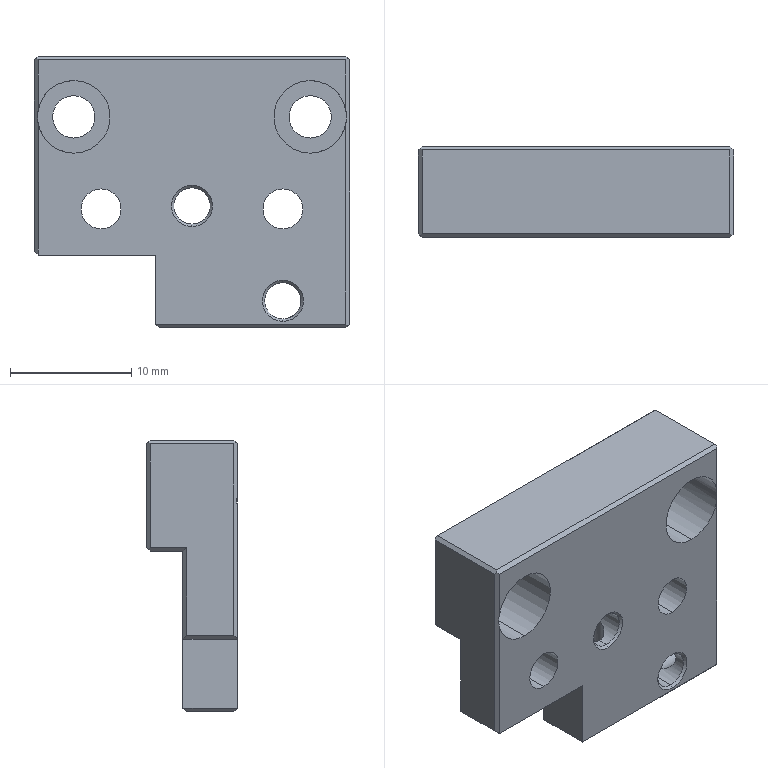Part | NX | 1 solid | 58 faces | box 26 x 7.5 x 22.4 mm | volume 2537 mm3 | plane 30 | cylinder 20 | cone 8 | commonest cylinder face diameters 2.5 x4 3 x4 3.3 x4 3.5 x4 6 x4